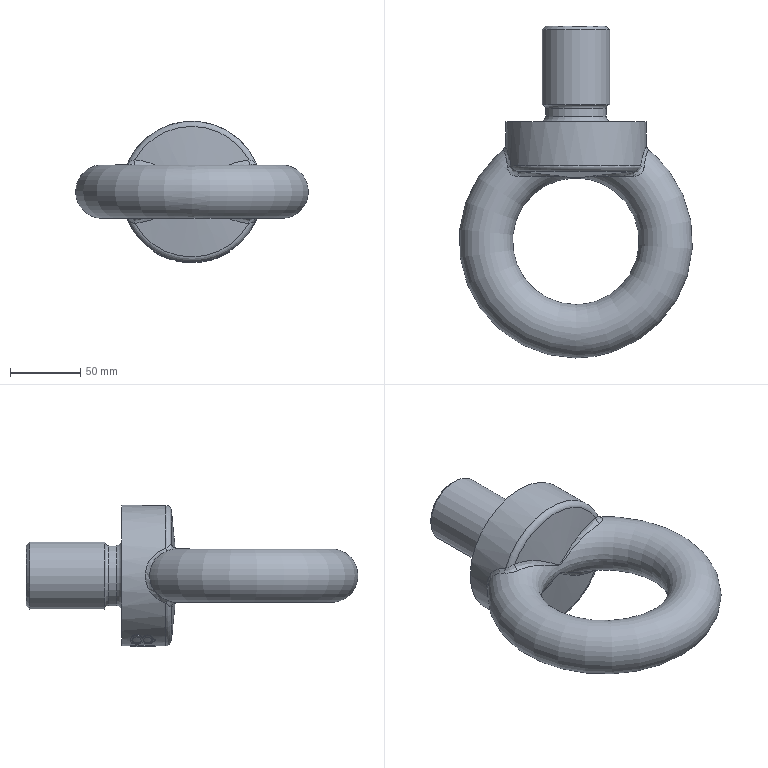Part | STEP file | solid 141 | 1 solid | 107 faces | box 166 x 236 x 100.5 mm | volume 770612 mm3 | other 75 | plane 8 | cylinder 8 | spline 8 | torus 5 | cone 3 | commonest cylinder face diameters 100 x3 101 x3 43 x1 48 x1